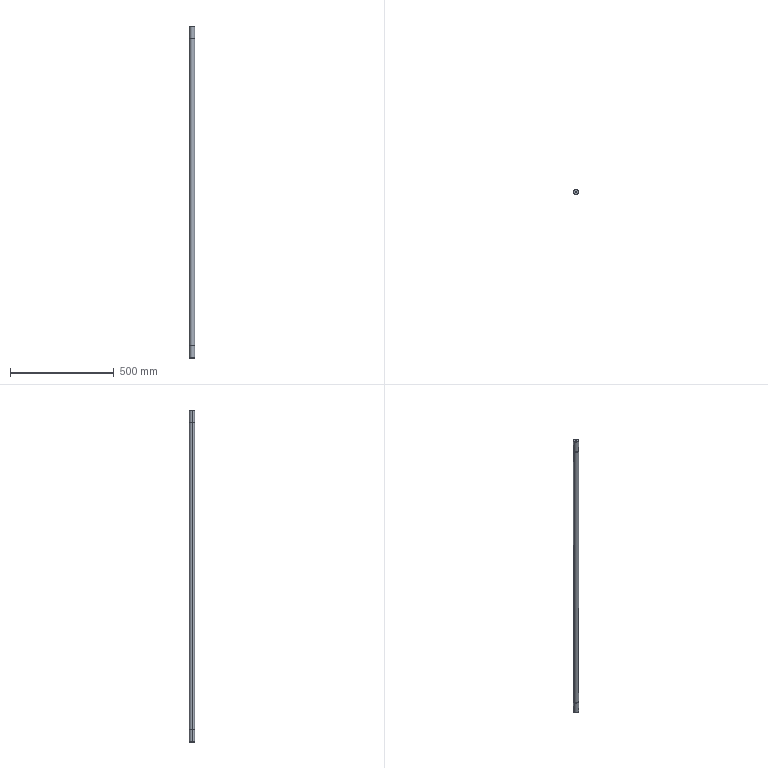Part | SolidWorks | features Chamfer 1, Extrusion 1, HoleWzd 1, MirrorPattern 1, RevCut 1 | 1 solid | 28 faces | box 25 x 25 x 1600 mm | volume 783785 mm3 | cylinder 14 | cone 8 | plane 6 | commonest cylinder face diameters 25 x6 6.8 x4 23.9 x4
STEP:
#1=CARTESIAN_POINT('',(3.4,0.,19.75));
#2=VERTEX_POINT('',#1);
#3=CARTESIAN_POINT('',(-3.4,0.,19.75));
#4=VERTEX_POINT('',#3);
#5=CARTESIAN_POINT('',(0.,0.,19.75));
#6=DIRECTION('',(0.,0.,-1.));
#7=DIRECTION('',(-1.,0.,0.));
#8=AXIS2_PLACEMENT_3D('',#5,#6,#7);
#9=CIRCLE('',#8,3.4);
#10=EDGE_CURVE('',#2,#4,#9,.T.);
#11=ORIENTED_EDGE('',*,*,#10,.F.);
#12=CARTESIAN_POINT('',(3.4,0.,0.));
#13=VERTEX_POINT('',#12);
#14=CARTESIAN_POINT('',(3.4,0.,0.));
#15=DIRECTION('',(0.,0.,-1.));
#16=VECTOR('',#15,1000.);
#17=LINE('',#14,#16);
#18=EDGE_CURVE('',#2,#13,#17,.T.);
#19=ORIENTED_EDGE('',*,*,#18,.T.);
#20=CARTESIAN_POINT('',(-3.4,0.,0.));
#21=VERTEX_POINT('',#20);
#22=CARTESIAN_POINT('',(0.,0.,0.));
#23=DIRECTION('',(0.,0.,-1.));
#24=DIRECTION('',(-1.,0.,0.));
#25=AXIS2_PLACEMENT_3D('',#22,#23,#24);
#26=CIRCLE('',#25,3.4);
#27=EDGE_CURVE('',#13,#21,#26,.T.);
#28=ORIENTED_EDGE('',*,*,#27,.T.);
#29=CARTESIAN_POINT('',(-3.4,0.,0.));
#30=DIRECTION('',(0.,0.,-1.));
#31=VECTOR('',#30,1000.);
#32=LINE('',#29,#31);
#33=EDGE_CURVE('',#4,#21,#32,.T.);
#34=ORIENTED_EDGE('',*,*,#33,.F.);
#35=EDGE_LOOP('',(#11,#19,#28,#34));
#36=FACE_OUTER_BOUND('',#35,.T.);
#37=CARTESIAN_POINT('',(0.,0.,0.));
#38=DIRECTION('',(0.,0.,-1.));
#39=DIRECTION('',(-1.,0.,0.));
#40=AXIS2_PLACEMENT_3D('',#37,#38,#39);
#41=CYLINDRICAL_SURFACE('',#40,3.4);
#42=ADVANCED_FACE('',(#36),#41,.F.);
#43=CARTESIAN_POINT('',(0.,0.,21.793));
#44=VERTEX_POINT('',#43);
#45=CARTESIAN_POINT('',(-3.4,0.,19.75));
#46=DIRECTION('',(-0.8572,0.,-0.515));
#47=VECTOR('',#46,1000.);
#48=LINE('',#45,#47);
#49=EDGE_CURVE('',#44,#4,#48,.T.);
#50=ORIENTED_EDGE('',*,*,#49,.F.);
#51=CARTESIAN_POINT('',(3.4,0.,19.75));
#52=DIRECTION('',(0.8572,0.,-0.515));
#53=VECTOR('',#52,1000.);
#54=LINE('',#51,#53);
#55=EDGE_CURVE('',#44,#2,#54,.T.);
#56=ORIENTED_EDGE('',*,*,#55,.T.);
#57=ORIENTED_EDGE('',*,*,#10,.T.);
#58=EDGE_LOOP('',(#50,#56,#57));
#59=FACE_OUTER_BOUND('',#58,.T.);
#60=CARTESIAN_POINT('',(0.,0.,19.75));
#61=DIRECTION('',(0.,0.,-1.));
#62=DIRECTION('',(-1.,0.,0.));
#63=AXIS2_PLACEMENT_3D('',#60,#61,#62);
#64=CONICAL_SURFACE('',#63,3.4,1.03);
#65=ADVANCED_FACE('',(#59),#64,.F.);
#66=CARTESIAN_POINT('',(12.5,0.,58.8));
#67=VERTEX_POINT('',#66);
#68=CARTESIAN_POINT('',(-12.5,0.,58.8));
#69=VERTEX_POINT('',#68);
#70=CARTESIAN_POINT('',(0.,0.,58.8));
#71=DIRECTION('',(0.,0.,1.));
#72=DIRECTION('',(1.,0.,0.));
#73=AXIS2_PLACEMENT_3D('',#70,#71,#72);
#74=CIRCLE('',#73,12.5);
#75=EDGE_CURVE('',#67,#69,#74,.T.);
#76=ORIENTED_EDGE('',*,*,#75,.F.);
#77=CARTESIAN_POINT('',(12.5,0.,0.5));
#78=VERTEX_POINT('',#77);
#79=CARTESIAN_POINT('',(12.5,0.,1600.));
#80=DIRECTION('',(0.,0.,-1.));
#81=VECTOR('',#80,1000.);
#82=LINE('',#79,#81);
#83=EDGE_CURVE('',#67,#78,#82,.T.);
#84=ORIENTED_EDGE('',*,*,#83,.T.);
#85=CARTESIAN_POINT('',(-12.5,0.,0.5));
#86=VERTEX_POINT('',#85);
#87=CARTESIAN_POINT('',(0.,0.,0.5));
#88=DIRECTION('',(0.,0.,1.));
#89=DIRECTION('',(1.,0.,0.));
#90=AXIS2_PLACEMENT_3D('',#87,#88,#89);
#91=CIRCLE('',#90,12.5);
#92=EDGE_CURVE('',#78,#86,#91,.T.);
#93=ORIENTED_EDGE('',*,*,#92,.T.);
#94=CARTESIAN_POINT('',(-12.5,0.,1600.));
#95=DIRECTION('',(0.,0.,-1.));
#96=VECTOR('',#95,1000.);
#97=LINE('',#94,#96);
#98=EDGE_CURVE('',#69,#86,#97,.T.);
#99=ORIENTED_EDGE('',*,*,#98,.F.);
#100=EDGE_LOOP('',(#76,#84,#93,#99));
#101=FACE_OUTER_BOUND('',#100,.T.);
#102=CARTESIAN_POINT('',(0.,0.,1600.));
#103=DIRECTION('',(0.,0.,-1.));
#104=DIRECTION('',(-1.,0.,0.));
#105=AXIS2_PLACEMENT_3D('',#102,#103,#104);
#106=CYLINDRICAL_SURFACE('',#105,12.5);
#107=ADVANCED_FACE('',(#101),#106,.T.);
#108=CARTESIAN_POINT('',(-12.,0.,0.));
#109=VERTEX_POINT('',#108);
#110=CARTESIAN_POINT('',(12.,0.,0.));
#111=VERTEX_POINT('',#110);
#112=CARTESIAN_POINT('',(0.,0.,0.));
#113=DIRECTION('',(0.,0.,-1.));
#114=DIRECTION('',(1.,0.,0.));
#115=AXIS2_PLACEMENT_3D('',#112,#113,#114);
#116=CIRCLE('',#115,12.);
#117=EDGE_CURVE('',#109,#111,#116,.T.);
#118=ORIENTED_EDGE('',*,*,#117,.F.);
#119=CARTESIAN_POINT('',(-12.5,0.,0.5));
#120=DIRECTION('',(-0.7071,0.,0.7071));
#121=VECTOR('',#120,1000.);
#122=LINE('',#119,#121);
#123=EDGE_CURVE('',#109,#86,#122,.T.);
#124=ORIENTED_EDGE('',*,*,#123,.T.);
#125=ORIENTED_EDGE('',*,*,#92,.F.);
#126=CARTESIAN_POINT('',(12.5,0.,0.5));
#127=DIRECTION('',(0.7071,0.,0.7071));
#128=VECTOR('',#127,1000.);
#129=LINE('',#126,#128);
#130=EDGE_CURVE('',#111,#78,#129,.T.);
#131=ORIENTED_EDGE('',*,*,#130,.F.);
#132=EDGE_LOOP('',(#118,#124,#125,#131));
#133=FACE_OUTER_BOUND('',#132,.T.);
#134=CARTESIAN_POINT('',(0.,0.,0.5));
#135=DIRECTION('',(0.,0.,1.));
#136=DIRECTION('',(1.,0.,0.));
#137=AXIS2_PLACEMENT_3D('',#134,#135,#136);
#138=CONICAL_SURFACE('',#137,12.5,0.7854);
#139=ADVANCED_FACE('',(#133),#138,.T.);
#140=CARTESIAN_POINT('',(-11.95,0.,60.1));
#141=VERTEX_POINT('',#140);
#142=CARTESIAN_POINT('',(11.95,0.,60.1));
#143=VERTEX_POINT('',#142);
#144=CARTESIAN_POINT('',(0.,0.,60.1));
#145=DIRECTION('',(0.,0.,1.));
#146=DIRECTION('',(1.,0.,0.));
#147=AXIS2_PLACEMENT_3D('',#144,#145,#146);
#148=CIRCLE('',#147,11.95);
#149=EDGE_CURVE('',#141,#143,#148,.T.);
#150=ORIENTED_EDGE('',*,*,#149,.F.);
#151=CARTESIAN_POINT('',(-11.95,0.,58.8));
#152=VERTEX_POINT('',#151);
#153=CARTESIAN_POINT('',(-11.95,0.,0.5));
#154=DIRECTION('',(0.,0.,-1.));
#155=VECTOR('',#154,1000.);
#156=LINE('',#153,#155);
#157=EDGE_CURVE('',#141,#152,#156,.T.);
#158=ORIENTED_EDGE('',*,*,#157,.T.);
#159=CARTESIAN_POINT('',(11.95,0.,58.8));
#160=VERTEX_POINT('',#159);
#161=CARTESIAN_POINT('',(0.,0.,58.8));
#162=DIRECTION('',(0.,0.,1.));
#163=DIRECTION('',(1.,0.,0.));
#164=AXIS2_PLACEMENT_3D('',#161,#162,#163);
#165=CIRCLE('',#164,11.95);
#166=EDGE_CURVE('',#152,#160,#165,.T.);
#167=ORIENTED_EDGE('',*,*,#166,.T.);
#168=CARTESIAN_POINT('',(11.95,0.,0.5));
#169=DIRECTION('',(0.,0.,-1.));
#170=VECTOR('',#169,1000.);
#171=LINE('',#168,#170);
#172=EDGE_CURVE('',#143,#160,#171,.T.);
#173=ORIENTED_EDGE('',*,*,#172,.F.);
#174=EDGE_LOOP('',(#150,#158,#167,#173));
#175=FACE_OUTER_BOUND('',#174,.T.);
#176=CARTESIAN_POINT('',(0.,0.,0.5));
#177=DIRECTION('',(0.,0.,-1.));
#178=DIRECTION('',(1.,0.,0.));
#179=AXIS2_PLACEMENT_3D('',#176,#177,#178);
#180=CYLINDRICAL_SURFACE('',#179,11.95);
#181=ADVANCED_FACE('',(#175),#180,.T.);
#182=CARTESIAN_POINT('',(-3.4,0.,1580.25));
#183=VERTEX_POINT('',#182);
#184=CARTESIAN_POINT('',(3.4,0.,1580.25));
#185=VERTEX_POINT('',#184);
#186=CARTESIAN_POINT('',(0.,0.,1580.25));
#187=DIRECTION('',(0.,0.,1.));
#188=DIRECTION('',(1.,0.,0.));
#189=AXIS2_PLACEMENT_3D('',#186,#187,#188);
#190=CIRCLE('',#189,3.4);
#191=EDGE_CURVE('',#183,#185,#190,.T.);
#192=ORIENTED_EDGE('',*,*,#191,.F.);
#193=CARTESIAN_POINT('',(-3.4,0.,1600.));
#194=VERTEX_POINT('',#193);
#195=CARTESIAN_POINT('',(-3.4,0.,1600.));
#196=DIRECTION('',(0.,0.,1.));
#197=VECTOR('',#196,1000.);
#198=LINE('',#195,#197);
#199=EDGE_CURVE('',#183,#194,#198,.T.);
#200=ORIENTED_EDGE('',*,*,#199,.T.);
#201=CARTESIAN_POINT('',(3.4,0.,1600.));
#202=VERTEX_POINT('',#201);
#203=CARTESIAN_POINT('',(0.,0.,1600.));
#204=DIRECTION('',(0.,0.,1.));
#205=DIRECTION('',(1.,0.,0.));
#206=AXIS2_PLACEMENT_3D('',#203,#204,#205);
#207=CIRCLE('',#206,3.4);
#208=EDGE_CURVE('',#194,#202,#207,.T.);
#209=ORIENTED_EDGE('',*,*,#208,.T.);
#210=CARTESIAN_POINT('',(3.4,0.,1600.));
#211=DIRECTION('',(0.,0.,1.));
#212=VECTOR('',#211,1000.);
#213=LINE('',#210,#212);
#214=EDGE_CURVE('',#185,#202,#213,.T.);
#215=ORIENTED_EDGE('',*,*,#214,.F.);
#216=EDGE_LOOP('',(#192,#200,#209,#215));
#217=FACE_OUTER_BOUND('',#216,.T.);
#218=CARTESIAN_POINT('',(0.,0.,1600.));
#219=DIRECTION('',(0.,0.,1.));
#220=DIRECTION('',(1.,0.,0.));
#221=AXIS2_PLACEMENT_3D('',#218,#219,#220);
#222=CYLINDRICAL_SURFACE('',#221,3.4);
#223=ADVANCED_FACE('',(#217),#222,.F.);
#224=CARTESIAN_POINT('',(0.,0.,1578.207));
#225=VERTEX_POINT('',#224);
#226=CARTESIAN_POINT('',(3.4,0.,1580.25));
#227=DIRECTION('',(0.8572,0.,0.515));
#228=VECTOR('',#227,1000.);
#229=LINE('',#226,#228);
#230=EDGE_CURVE('',#225,#185,#229,.T.);
#231=ORIENTED_EDGE('',*,*,#230,.F.);
#232=CARTESIAN_POINT('',(-3.4,0.,1580.25));
#233=DIRECTION('',(-0.8572,0.,0.515));
#234=VECTOR('',#233,1000.);
#235=LINE('',#232,#234);
#236=EDGE_CURVE('',#225,#183,#235,.T.);
#237=ORIENTED_EDGE('',*,*,#236,.T.);
#238=ORIENTED_EDGE('',*,*,#191,.T.);
#239=EDGE_LOOP('',(#231,#237,#238));
#240=FACE_OUTER_BOUND('',#239,.T.);
#241=CARTESIAN_POINT('',(0.,0.,1580.25));
#242=DIRECTION('',(0.,0.,1.));
#243=DIRECTION('',(1.,0.,0.));
#244=AXIS2_PLACEMENT_3D('',#241,#242,#243);
#245=CONICAL_SURFACE('',#244,3.4,1.03);
#246=ADVANCED_FACE('',(#240),#245,.F.);
#247=CARTESIAN_POINT('',(12.5,0.,1539.9));
#248=VERTEX_POINT('',#247);
#249=CARTESIAN_POINT('',(-12.5,0.,1539.9));
#250=VERTEX_POINT('',#249);
#251=CARTESIAN_POINT('',(0.,0.,1539.9));
#252=DIRECTION('',(0.,0.,1.));
#253=DIRECTION('',(1.,0.,0.));
#254=AXIS2_PLACEMENT_3D('',#251,#252,#253);
#255=CIRCLE('',#254,12.5);
#256=EDGE_CURVE('',#248,#250,#255,.T.);
#257=ORIENTED_EDGE('',*,*,#256,.F.);
#258=CARTESIAN_POINT('',(12.5,0.,60.1));
#259=VERTEX_POINT('',#258);
#260=CARTESIAN_POINT('',(12.5,0.,1600.));
#261=DIRECTION('',(0.,0.,-1.));
#262=VECTOR('',#261,1000.);
#263=LINE('',#260,#262);
#264=EDGE_CURVE('',#248,#259,#263,.T.);
#265=ORIENTED_EDGE('',*,*,#264,.T.);
#266=CARTESIAN_POINT('',(-12.5,0.,60.1));
#267=VERTEX_POINT('',#266);
#268=CARTESIAN_POINT('',(0.,0.,60.1));
#269=DIRECTION('',(0.,0.,1.));
#270=DIRECTION('',(1.,0.,0.));
#271=AXIS2_PLACEMENT_3D('',#268,#269,#270);
#272=CIRCLE('',#271,12.5);
#273=EDGE_CURVE('',#259,#267,#272,.T.);
#274=ORIENTED_EDGE('',*,*,#273,.T.);
#275=CARTESIAN_POINT('',(-12.5,0.,1600.));
#276=DIRECTION('',(0.,0.,-1.));
#277=VECTOR('',#276,1000.);
#278=LINE('',#275,#277);
#279=EDGE_CURVE('',#250,#267,#278,.T.);
#280=ORIENTED_EDGE('',*,*,#279,.F.);
#281=EDGE_LOOP('',(#257,#265,#274,#280));
#282=FACE_OUTER_BOUND('',#281,.T.);
#283=CARTESIAN_POINT('',(0.,0.,1600.));
#284=DIRECTION('',(0.,0.,-1.));
#285=DIRECTION('',(-1.,0.,0.));
#286=AXIS2_PLACEMENT_3D('',#283,#284,#285);
#287=CYLINDRICAL_SURFACE('',#286,12.5);
#288=ADVANCED_FACE('',(#282),#287,.T.);
#289=CARTESIAN_POINT('',(11.95,0.,1539.9));
#290=VERTEX_POINT('',#289);
#291=CARTESIAN_POINT('',(-11.95,0.,1539.9));
#292=VERTEX_POINT('',#291);
#293=CARTESIAN_POINT('',(0.,0.,1539.9));
#294=DIRECTION('',(0.,0.,1.));
#295=DIRECTION('',(1.,0.,0.));
#296=AXIS2_PLACEMENT_3D('',#293,#294,#295);
#297=CIRCLE('',#296,11.95);
#298=EDGE_CURVE('',#290,#292,#297,.T.);
#299=ORIENTED_EDGE('',*,*,#298,.T.);
#300=CARTESIAN_POINT('',(-11.95,0.,1541.2));
#301=VERTEX_POINT('',#300);
#302=CARTESIAN_POINT('',(-11.95,0.,1599.5));
#303=DIRECTION('',(0.,0.,1.));
#304=VECTOR('',#303,1000.);
#305=LINE('',#302,#304);
#306=EDGE_CURVE('',#292,#301,#305,.T.);
#307=ORIENTED_EDGE('',*,*,#306,.T.);
#308=CARTESIAN_POINT('',(11.95,0.,1541.2));
#309=VERTEX_POINT('',#308);
#310=CARTESIAN_POINT('',(0.,0.,1541.2));
#311=DIRECTION('',(0.,0.,1.));
#312=DIRECTION('',(1.,0.,0.));
#313=AXIS2_PLACEMENT_3D('',#310,#311,#312);
#314=CIRCLE('',#313,11.95);
#315=EDGE_CURVE('',#309,#301,#314,.T.);
#316=ORIENTED_EDGE('',*,*,#315,.F.);
#317=CARTESIAN_POINT('',(11.95,0.,1599.5));
#318=DIRECTION('',(0.,0.,1.));
#319=VECTOR('',#318,1000.);
#320=LINE('',#317,#319);
#321=EDGE_CURVE('',#290,#309,#320,.T.);
#322=ORIENTED_EDGE('',*,*,#321,.F.);
#323=EDGE_LOOP('',(#299,#307,#316,#322));
#324=FACE_OUTER_BOUND('',#323,.T.);
#325=CARTESIAN_POINT('',(0.,0.,1599.5));
#326=DIRECTION('',(0.,0.,1.));
#327=DIRECTION('',(1.,0.,0.));
#328=AXIS2_PLACEMENT_3D('',#325,#326,#327);
#329=CYLINDRICAL_SURFACE('',#328,11.95);
#330=ADVANCED_FACE('',(#324),#329,.T.);
#331=CARTESIAN_POINT('',(12.,0.,1600.));
#332=VERTEX_POINT('',#331);
#333=CARTESIAN_POINT('',(-12.,0.,1600.));
#334=VERTEX_POINT('',#333);
#335=CARTESIAN_POINT('',(0.,0.,1600.));
#336=DIRECTION('',(0.,0.,1.));
#337=DIRECTION('',(1.,0.,0.));
#338=AXIS2_PLACEMENT_3D('',#335,#336,#337);
#339=CIRCLE('',#338,12.);
#340=EDGE_CURVE('',#332,#334,#339,.T.);
#341=ORIENTED_EDGE('',*,*,#340,.F.);
#342=CARTESIAN_POINT('',(12.5,0.,1599.5));
#343=VERTEX_POINT('',#342);
#344=CARTESIAN_POINT('',(12.,0.,1600.));
#345=DIRECTION('',(0.7071,0.,-0.7071));
#346=VECTOR('',#345,1000.);
#347=LINE('',#344,#346);
#348=EDGE_CURVE('',#332,#343,#347,.T.);
#349=ORIENTED_EDGE('',*,*,#348,.T.);
#350=CARTESIAN_POINT('',(-12.5,0.,1599.5));
#351=VERTEX_POINT('',#350);
#352=CARTESIAN_POINT('',(0.,0.,1599.5));
#353=DIRECTION('',(0.,0.,-1.));
#354=DIRECTION('',(1.,0.,0.));
#355=AXIS2_PLACEMENT_3D('',#352,#353,#354);
#356=CIRCLE('',#355,12.5);
#357=EDGE_CURVE('',#351,#343,#356,.T.);
#358=ORIENTED_EDGE('',*,*,#357,.F.);
#359=CARTESIAN_POINT('',(-12.,0.,1600.));
#360=DIRECTION('',(-0.7071,0.,-0.7071));
#361=VECTOR('',#360,1000.);
#362=LINE('',#359,#361);
#363=EDGE_CURVE('',#334,#351,#362,.T.);
#364=ORIENTED_EDGE('',*,*,#363,.F.);
#365=EDGE_LOOP('',(#341,#349,#358,#364));
#366=FACE_OUTER_BOUND('',#365,.T.);
#367=CARTESIAN_POINT('',(0.,0.,1600.));
#368=DIRECTION('',(0.,0.,-1.));
#369=DIRECTION('',(-1.,0.,0.));
#370=AXIS2_PLACEMENT_3D('',#367,#368,#369);
#371=CONICAL_SURFACE('',#370,12.,0.7854);
#372=ADVANCED_FACE('',(#366),#371,.T.);
#373=ORIENTED_EDGE('',*,*,#357,.T.);
#374=CARTESIAN_POINT('',(12.5,0.,1541.2));
#375=VERTEX_POINT('',#374);
#376=CARTESIAN_POINT('',(12.5,0.,1600.));
#377=DIRECTION('',(0.,0.,-1.));
#378=VECTOR('',#377,1000.);
#379=LINE('',#376,#378);
#380=EDGE_CURVE('',#343,#375,#379,.T.);
#381=ORIENTED_EDGE('',*,*,#380,.T.);
#382=CARTESIAN_POINT('',(-12.5,0.,1541.2));
#383=VERTEX_POINT('',#382);
#384=CARTESIAN_POINT('',(0.,0.,1541.2));
#385=DIRECTION('',(0.,0.,1.));
#386=DIRECTION('',(1.,0.,0.));
#387=AXIS2_PLACEMENT_3D('',#384,#385,#386);
#388=CIRCLE('',#387,12.5);
#389=EDGE_CURVE('',#375,#383,#388,.T.);
#390=ORIENTED_EDGE('',*,*,#389,.T.);
#391=CARTESIAN_POINT('',(-12.5,0.,1600.));
#392=DIRECTION('',(0.,0.,-1.));
#393=VECTOR('',#392,1000.);
#394=LINE('',#391,#393);
#395=EDGE_CURVE('',#351,#383,#394,.T.);
#396=ORIENTED_EDGE('',*,*,#395,.F.);
#397=EDGE_LOOP('',(#373,#381,#390,#396));
#398=FACE_OUTER_BOUND('',#397,.T.);
#399=CARTESIAN_POINT('',(0.,0.,1600.));
#400=DIRECTION('',(0.,0.,-1.));
#401=DIRECTION('',(-1.,0.,0.));
#402=AXIS2_PLACEMENT_3D('',#399,#400,#401);
#403=CYLINDRICAL_SURFACE('',#402,12.5);
#404=ADVANCED_FACE('',(#398),#403,.T.);
#405=ORIENTED_EDGE('',*,*,#380,.F.);
#406=CARTESIAN_POINT('',(0.,0.,1599.5));
#407=DIRECTION('',(0.,0.,-1.));
#408=DIRECTION('',(1.,0.,0.));
#409=AXIS2_PLACEMENT_3D('',#406,#407,#408);
#410=CIRCLE('',#409,12.5);
#411=EDGE_CURVE('',#343,#351,#410,.T.);
#412=ORIENTED_EDGE('',*,*,#411,.T.);
#413=ORIENTED_EDGE('',*,*,#395,.T.);
#414=CARTESIAN_POINT('',(0.,0.,1541.2));
#415=DIRECTION('',(0.,0.,1.));
#416=DIRECTION('',(1.,0.,0.));
#417=AXIS2_PLACEMENT_3D('',#414,#415,#416);
#418=CIRCLE('',#417,12.5);
#419=EDGE_CURVE('',#383,#375,#418,.T.);
#420=ORIENTED_EDGE('',*,*,#419,.T.);
#421=EDGE_LOOP('',(#405,#412,#413,#420));
#422=FACE_OUTER_BOUND('',#421,.T.);
#423=CARTESIAN_POINT('',(0.,0.,1600.));
#424=DIRECTION('',(0.,0.,-1.));
#425=DIRECTION('',(-1.,0.,0.));
#426=AXIS2_PLACEMENT_3D('',#423,#424,#425);
#427=CYLINDRICAL_SURFACE('',#426,12.5);
#428=ADVANCED_FACE('',(#422),#427,.T.);
#429=CARTESIAN_POINT('',(0.,0.,1600.));
#430=DIRECTION('',(0.,0.,1.));
#431=DIRECTION('',(1.,0.,0.));
#432=AXIS2_PLACEMENT_3D('',#429,#430,#431);
#433=CIRCLE('',#432,3.4);
#434=EDGE_CURVE('',#202,#194,#433,.T.);
#435=ORIENTED_EDGE('',*,*,#434,.F.);
#436=ORIENTED_EDGE('',*,*,#208,.F.);
#437=EDGE_LOOP('',(#435,#436));
#438=FACE_BOUND('',#437,.T.);
#439=CARTESIAN_POINT('',(0.,0.,1600.));
#440=DIRECTION('',(0.,0.,1.));
#441=DIRECTION('',(1.,0.,0.));
#442=AXIS2_PLACEMENT_3D('',#439,#440,#441);
#443=CIRCLE('',#442,12.);
#444=EDGE_CURVE('',#334,#332,#443,.T.);
#445=ORIENTED_EDGE('',*,*,#444,.T.);
#446=ORIENTED_EDGE('',*,*,#340,.T.);
#447=EDGE_LOOP('',(#445,#446));
#448=FACE_OUTER_BOUND('',#447,.T.);
#449=CARTESIAN_POINT('',(0.,0.,1600.));
#450=DIRECTION('',(0.,0.,1.));
#451=DIRECTION('',(1.,0.,0.));
#452=AXIS2_PLACEMENT_3D('',#449,#450,#451);
#453=PLANE('',#452);
#454=ADVANCED_FACE('',(#438,#448),#453,.T.);
#455=ORIENTED_EDGE('',*,*,#348,.F.);
#456=ORIENTED_EDGE('',*,*,#444,.F.);
#457=ORIENTED_EDGE('',*,*,#363,.T.);
#458=ORIENTED_EDGE('',*,*,#411,.F.);
#459=EDGE_LOOP('',(#455,#456,#457,#458));
#460=FACE_OUTER_BOUND('',#459,.T.);
#461=CARTESIAN_POINT('',(0.,0.,1600.));
#462=DIRECTION('',(0.,0.,-1.));
#463=DIRECTION('',(-1.,0.,0.));
#464=AXIS2_PLACEMENT_3D('',#461,#462,#463);
#465=CONICAL_SURFACE('',#464,12.,0.7854);
#466=ADVANCED_FACE('',(#460),#465,.T.);
#467=ORIENTED_EDGE('',*,*,#419,.F.);
#468=ORIENTED_EDGE('',*,*,#389,.F.);
#469=EDGE_LOOP('',(#467,#468));
#470=FACE_OUTER_BOUND('',#469,.T.);
#471=ORIENTED_EDGE('',*,*,#315,.T.);
#472=CARTESIAN_POINT('',(0.,0.,1541.2));
#473=DIRECTION('',(0.,0.,1.));
#474=DIRECTION('',(1.,0.,0.));
#475=AXIS2_PLACEMENT_3D('',#472,#473,#474);
#476=CIRCLE('',#475,11.95);
#477=EDGE_CURVE('',#301,#309,#476,.T.);
#478=ORIENTED_EDGE('',*,*,#477,.T.);
#479=EDGE_LOOP('',(#471,#478));
#480=FACE_BOUND('',#479,.T.);
#481=CARTESIAN_POINT('',(12.5,0.,1541.2));
#482=DIRECTION('',(0.,0.,1.));
#483=DIRECTION('',(1.,0.,0.));
#484=AXIS2_PLACEMENT_3D('',#481,#482,#483);
#485=PLANE('',#484);
#486=ADVANCED_FACE('',(#470,#480),#485,.F.);
#487=ORIENTED_EDGE('',*,*,#306,.F.);
#488=CARTESIAN_POINT('',(0.,0.,1539.9));
#489=DIRECTION('',(0.,0.,1.));
#490=DIRECTION('',(1.,0.,0.));
#491=AXIS2_PLACEMENT_3D('',#488,#489,#490);
#492=CIRCLE('',#491,11.95);
#493=EDGE_CURVE('',#292,#290,#492,.T.);
#494=ORIENTED_EDGE('',*,*,#493,.T.);
#495=ORIENTED_EDGE('',*,*,#321,.T.);
#496=ORIENTED_EDGE('',*,*,#477,.F.);
#497=EDGE_LOOP('',(#487,#494,#495,#496));
#498=FACE_OUTER_BOUND('',#497,.T.);
#499=CARTESIAN_POINT('',(0.,0.,1599.5));
#500=DIRECTION('',(0.,0.,1.));
#501=DIRECTION('',(1.,0.,0.));
#502=AXIS2_PLACEMENT_3D('',#499,#500,#501);
#503=CYLINDRICAL_SURFACE('',#502,11.95);
#504=ADVANCED_FACE('',(#498),#503,.T.);
#505=ORIENTED_EDGE('',*,*,#298,.F.);
#506=ORIENTED_EDGE('',*,*,#493,.F.);
#507=EDGE_LOOP('',(#505,#506));
#508=FACE_BOUND('',#507,.T.);
#509=CARTESIAN_POINT('',(0.,0.,1539.9));
#510=DIRECTION('',(0.,0.,1.));
#511=DIRECTION('',(1.,0.,0.));
#512=AXIS2_PLACEMENT_3D('',#509,#510,#511);
#513=CIRCLE('',#512,12.5);
#514=EDGE_CURVE('',#250,#248,#513,.T.);
#515=ORIENTED_EDGE('',*,*,#514,.T.);
#516=ORIENTED_EDGE('',*,*,#256,.T.);
#517=EDGE_LOOP('',(#515,#516));
#518=FACE_OUTER_BOUND('',#517,.T.);
#519=CARTESIAN_POINT('',(12.5,0.,1539.9));
#520=DIRECTION('',(0.,0.,-1.));
#521=DIRECTION('',(-1.,0.,0.));
#522=AXIS2_PLACEMENT_3D('',#519,#520,#521);
#523=PLANE('',#522);
#524=ADVANCED_FACE('',(#508,#518),#523,.F.);
#525=ORIENTED_EDGE('',*,*,#264,.F.);
#526=ORIENTED_EDGE('',*,*,#514,.F.);
#527=ORIENTED_EDGE('',*,*,#279,.T.);
#528=CARTESIAN_POINT('',(0.,0.,60.1));
#529=DIRECTION('',(0.,0.,1.));
#530=DIRECTION('',(1.,0.,0.));
#531=AXIS2_PLACEMENT_3D('',#528,#529,#530);
#532=CIRCLE('',#531,12.5);
#533=EDGE_CURVE('',#267,#259,#532,.T.);
#534=ORIENTED_EDGE('',*,*,#533,.T.);
#535=EDGE_LOOP('',(#525,#526,#527,#534));
#536=FACE_OUTER_BOUND('',#535,.T.);
#537=CARTESIAN_POINT('',(0.,0.,1600.));
#538=DIRECTION('',(0.,0.,-1.));
#539=DIRECTION('',(-1.,0.,0.));
#540=AXIS2_PLACEMENT_3D('',#537,#538,#539);
#541=CYLINDRICAL_SURFACE('',#540,12.5);
#542=ADVANCED_FACE('',(#536),#541,.T.);
#543=ORIENTED_EDGE('',*,*,#236,.F.);
#544=ORIENTED_EDGE('',*,*,#230,.T.);
#545=CARTESIAN_POINT('',(0.,0.,1580.25));
#546=DIRECTION('',(0.,0.,1.));
#547=DIRECTION('',(1.,0.,0.));
#548=AXIS2_PLACEMENT_3D('',#545,#546,#547);
#549=CIRCLE('',#548,3.4);
#550=EDGE_CURVE('',#185,#183,#549,.T.);
#551=ORIENTED_EDGE('',*,*,#550,.T.);
#552=EDGE_LOOP('',(#543,#544,#551));
#553=FACE_OUTER_BOUND('',#552,.T.);
#554=CARTESIAN_POINT('',(0.,0.,1580.25));
#555=DIRECTION('',(0.,0.,1.));
#556=DIRECTION('',(1.,0.,0.));
#557=AXIS2_PLACEMENT_3D('',#554,#555,#556);
#558=CONICAL_SURFACE('',#557,3.4,1.03);
#559=ADVANCED_FACE('',(#553),#558,.F.);
#560=ORIENTED_EDGE('',*,*,#199,.F.);
#561=ORIENTED_EDGE('',*,*,#550,.F.);
#562=ORIENTED_EDGE('',*,*,#214,.T.);
#563=ORIENTED_EDGE('',*,*,#434,.T.);
#564=EDGE_LOOP('',(#560,#561,#562,#563));
#565=FACE_OUTER_BOUND('',#564,.T.);
#566=CARTESIAN_POINT('',(0.,0.,1600.));
#567=DIRECTION('',(0.,0.,1.));
#568=DIRECTION('',(1.,0.,0.));
#569=AXIS2_PLACEMENT_3D('',#566,#567,#568);
#570=CYLINDRICAL_SURFACE('',#569,3.4);
#571=ADVANCED_FACE('',(#565),#570,.F.);
#572=CARTESIAN_POINT('',(0.,0.,58.8));
#573=DIRECTION('',(0.,0.,1.));
#574=DIRECTION('',(1.,0.,0.));
#575=AXIS2_PLACEMENT_3D('',#572,#573,#574);
#576=CIRCLE('',#575,12.5);
#577=EDGE_CURVE('',#69,#67,#576,.T.);
#578=ORIENTED_EDGE('',*,*,#577,.T.);
#579=ORIENTED_EDGE('',*,*,#75,.T.);
#580=EDGE_LOOP('',(#578,#579));
#581=FACE_OUTER_BOUND('',#580,.T.);
#582=CARTESIAN_POINT('',(0.,0.,58.8));
#583=DIRECTION('',(0.,0.,1.));
#584=DIRECTION('',(1.,0.,0.));
#585=AXIS2_PLACEMENT_3D('',#582,#583,#584);
#586=CIRCLE('',#585,11.95);
#587=EDGE_CURVE('',#160,#152,#586,.T.);
#588=ORIENTED_EDGE('',*,*,#587,.F.);
#589=ORIENTED_EDGE('',*,*,#166,.F.);
#590=EDGE_LOOP('',(#588,#589));
#591=FACE_BOUND('',#590,.T.);
#592=CARTESIAN_POINT('',(12.5,0.,58.8));
#593=DIRECTION('',(0.,0.,-1.));
#594=DIRECTION('',(1.,0.,0.));
#595=AXIS2_PLACEMENT_3D('',#592,#593,#594);
#596=PLANE('',#595);
#597=ADVANCED_FACE('',(#581,#591),#596,.F.);
#598=ORIENTED_EDGE('',*,*,#157,.F.);
#599=CARTESIAN_POINT('',(0.,0.,60.1));
#600=DIRECTION('',(0.,0.,1.));
#601=DIRECTION('',(1.,0.,0.));
#602=AXIS2_PLACEMENT_3D('',#599,#600,#601);
#603=CIRCLE('',#602,11.95);
#604=EDGE_CURVE('',#143,#141,#603,.T.);
#605=ORIENTED_EDGE('',*,*,#604,.F.);
#606=ORIENTED_EDGE('',*,*,#172,.T.);
#607=ORIENTED_EDGE('',*,*,#587,.T.);
#608=EDGE_LOOP('',(#598,#605,#606,#607));
#609=FACE_OUTER_BOUND('',#608,.T.);
#610=CARTESIAN_POINT('',(0.,0.,0.5));
#611=DIRECTION('',(0.,0.,-1.));
#612=DIRECTION('',(1.,0.,0.));
#613=AXIS2_PLACEMENT_3D('',#610,#611,#612);
#614=CYLINDRICAL_SURFACE('',#613,11.95);
#615=ADVANCED_FACE('',(#609),#614,.T.);
#616=ORIENTED_EDGE('',*,*,#604,.T.);
#617=ORIENTED_EDGE('',*,*,#149,.T.);
#618=EDGE_LOOP('',(#616,#617));
#619=FACE_BOUND('',#618,.T.);
#620=ORIENTED_EDGE('',*,*,#533,.F.);
#621=ORIENTED_EDGE('',*,*,#273,.F.);
#622=EDGE_LOOP('',(#620,#621));
#623=FACE_OUTER_BOUND('',#622,.T.);
#624=CARTESIAN_POINT('',(12.5,0.,60.1));
#625=DIRECTION('',(0.,0.,1.));
#626=DIRECTION('',(-1.,0.,0.));
#627=AXIS2_PLACEMENT_3D('',#624,#625,#626);
#628=PLANE('',#627);
#629=ADVANCED_FACE('',(#619,#623),#628,.F.);
#630=CARTESIAN_POINT('',(0.,0.,0.));
#631=DIRECTION('',(0.,0.,-1.));
#632=DIRECTION('',(-1.,0.,0.));
#633=AXIS2_PLACEMENT_3D('',#630,#631,#632);
#634=CIRCLE('',#633,3.4);
#635=EDGE_CURVE('',#21,#13,#634,.T.);
#636=ORIENTED_EDGE('',*,*,#635,.F.);
#637=ORIENTED_EDGE('',*,*,#27,.F.);
#638=EDGE_LOOP('',(#636,#637));
#639=FACE_BOUND('',#638,.T.);
#640=CARTESIAN_POINT('',(0.,0.,0.));
#641=DIRECTION('',(0.,0.,-1.));
#642=DIRECTION('',(1.,0.,0.));
#643=AXIS2_PLACEMENT_3D('',#640,#641,#642);
#644=CIRCLE('',#643,12.);
#645=EDGE_CURVE('',#111,#109,#644,.T.);
#646=ORIENTED_EDGE('',*,*,#645,.T.);
#647=ORIENTED_EDGE('',*,*,#117,.T.);
#648=EDGE_LOOP('',(#646,#647));
#649=FACE_OUTER_BOUND('',#648,.T.);
#650=CARTESIAN_POINT('',(0.,0.,0.));
#651=DIRECTION('',(0.,0.,1.));
#652=DIRECTION('',(1.,0.,0.));
#653=AXIS2_PLACEMENT_3D('',#650,#651,#652);
#654=PLANE('',#653);
#655=ADVANCED_FACE('',(#639,#649),#654,.F.);
#656=ORIENTED_EDGE('',*,*,#123,.F.);
#657=ORIENTED_EDGE('',*,*,#645,.F.);
#658=ORIENTED_EDGE('',*,*,#130,.T.);
#659=CARTESIAN_POINT('',(0.,0.,0.5));
#660=DIRECTION('',(0.,0.,1.));
#661=DIRECTION('',(1.,0.,0.));
#662=AXIS2_PLACEMENT_3D('',#659,#660,#661);
#663=CIRCLE('',#662,12.5);
#664=EDGE_CURVE('',#86,#78,#663,.T.);
#665=ORIENTED_EDGE('',*,*,#664,.F.);
#666=EDGE_LOOP('',(#656,#657,#658,#665));
#667=FACE_OUTER_BOUND('',#666,.T.);
#668=CARTESIAN_POINT('',(0.,0.,0.5));
#669=DIRECTION('',(0.,0.,1.));
#670=DIRECTION('',(1.,0.,0.));
#671=AXIS2_PLACEMENT_3D('',#668,#669,#670);
#672=CONICAL_SURFACE('',#671,12.5,0.7854);
#673=ADVANCED_FACE('',(#667),#672,.T.);
#674=ORIENTED_EDGE('',*,*,#83,.F.);
#675=ORIENTED_EDGE('',*,*,#577,.F.);
#676=ORIENTED_EDGE('',*,*,#98,.T.);
#677=ORIENTED_EDGE('',*,*,#664,.T.);
#678=EDGE_LOOP('',(#674,#675,#676,#677));
#679=FACE_OUTER_BOUND('',#678,.T.);
#680=CARTESIAN_POINT('',(0.,0.,1600.));
#681=DIRECTION('',(0.,0.,-1.));
#682=DIRECTION('',(-1.,0.,0.));
#683=AXIS2_PLACEMENT_3D('',#680,#681,#682);
#684=CYLINDRICAL_SURFACE('',#683,12.5);
#685=ADVANCED_FACE('',(#679),#684,.T.);
#686=ORIENTED_EDGE('',*,*,#55,.F.);
#687=ORIENTED_EDGE('',*,*,#49,.T.);
#688=CARTESIAN_POINT('',(0.,0.,19.75));
#689=DIRECTION('',(0.,0.,-1.));
#690=DIRECTION('',(-1.,0.,0.));
#691=AXIS2_PLACEMENT_3D('',#688,#689,#690);
#692=CIRCLE('',#691,3.4);
#693=EDGE_CURVE('',#4,#2,#692,.T.);
#694=ORIENTED_EDGE('',*,*,#693,.T.);
#695=EDGE_LOOP('',(#686,#687,#694));
#696=FACE_OUTER_BOUND('',#695,.T.);
#697=CARTESIAN_POINT('',(0.,0.,19.75));
#698=DIRECTION('',(0.,0.,-1.));
#699=DIRECTION('',(-1.,0.,0.));
#700=AXIS2_PLACEMENT_3D('',#697,#698,#699);
#701=CONICAL_SURFACE('',#700,3.4,1.03);
#702=ADVANCED_FACE('',(#696),#701,.F.);
#703=ORIENTED_EDGE('',*,*,#18,.F.);
#704=ORIENTED_EDGE('',*,*,#693,.F.);
#705=ORIENTED_EDGE('',*,*,#33,.T.);
#706=ORIENTED_EDGE('',*,*,#635,.T.);
#707=EDGE_LOOP('',(#703,#704,#705,#706));
#708=FACE_OUTER_BOUND('',#707,.T.);
#709=CARTESIAN_POINT('',(0.,0.,0.));
#710=DIRECTION('',(0.,0.,-1.));
#711=DIRECTION('',(-1.,0.,0.));
#712=AXIS2_PLACEMENT_3D('',#709,#710,#711);
#713=CYLINDRICAL_SURFACE('',#712,3.4);
#714=ADVANCED_FACE('',(#708),#713,.F.);
#715=CLOSED_SHELL('',(#42,#65,#107,#139,#181,#223,#246,#288,#330,#372,#404,#428,#454,#466,#486,#504,#524,#542,#559,#571,#597,#615,#629,#655,#673,#685,#702,#714));
#716=MANIFOLD_SOLID_BREP('',#715);
#717=CARTESIAN_POINT('',(0.,0.,0.));
#718=DIRECTION('',(0.,0.,1.));
#719=DIRECTION('',(1.,0.,0.));
#720=AXIS2_PLACEMENT_3D('',#717,#718,#719);
#721=(LENGTH_UNIT()NAMED_UNIT(*)SI_UNIT(.MILLI.,.METRE.));
#722=UNCERTAINTY_MEASURE_WITH_UNIT(LENGTH_MEASURE(0.00001),#721,'','');
#723=(NAMED_UNIT(*)PLANE_ANGLE_UNIT()SI_UNIT($,.RADIAN.));
#724=(NAMED_UNIT(*)SI_UNIT($,.STERADIAN.)SOLID_ANGLE_UNIT());
#725=(GEOMETRIC_REPRESENTATION_CONTEXT(3)GLOBAL_UNCERTAINTY_ASSIGNED_CONTEXT((#722))GLOBAL_UNIT_ASSIGNED_CONTEXT((#721,#723,#724))REPRESENTATION_CONTEXT('',''));
#726=ADVANCED_BREP_SHAPE_REPRESENTATION('',(#716,#720),#725);